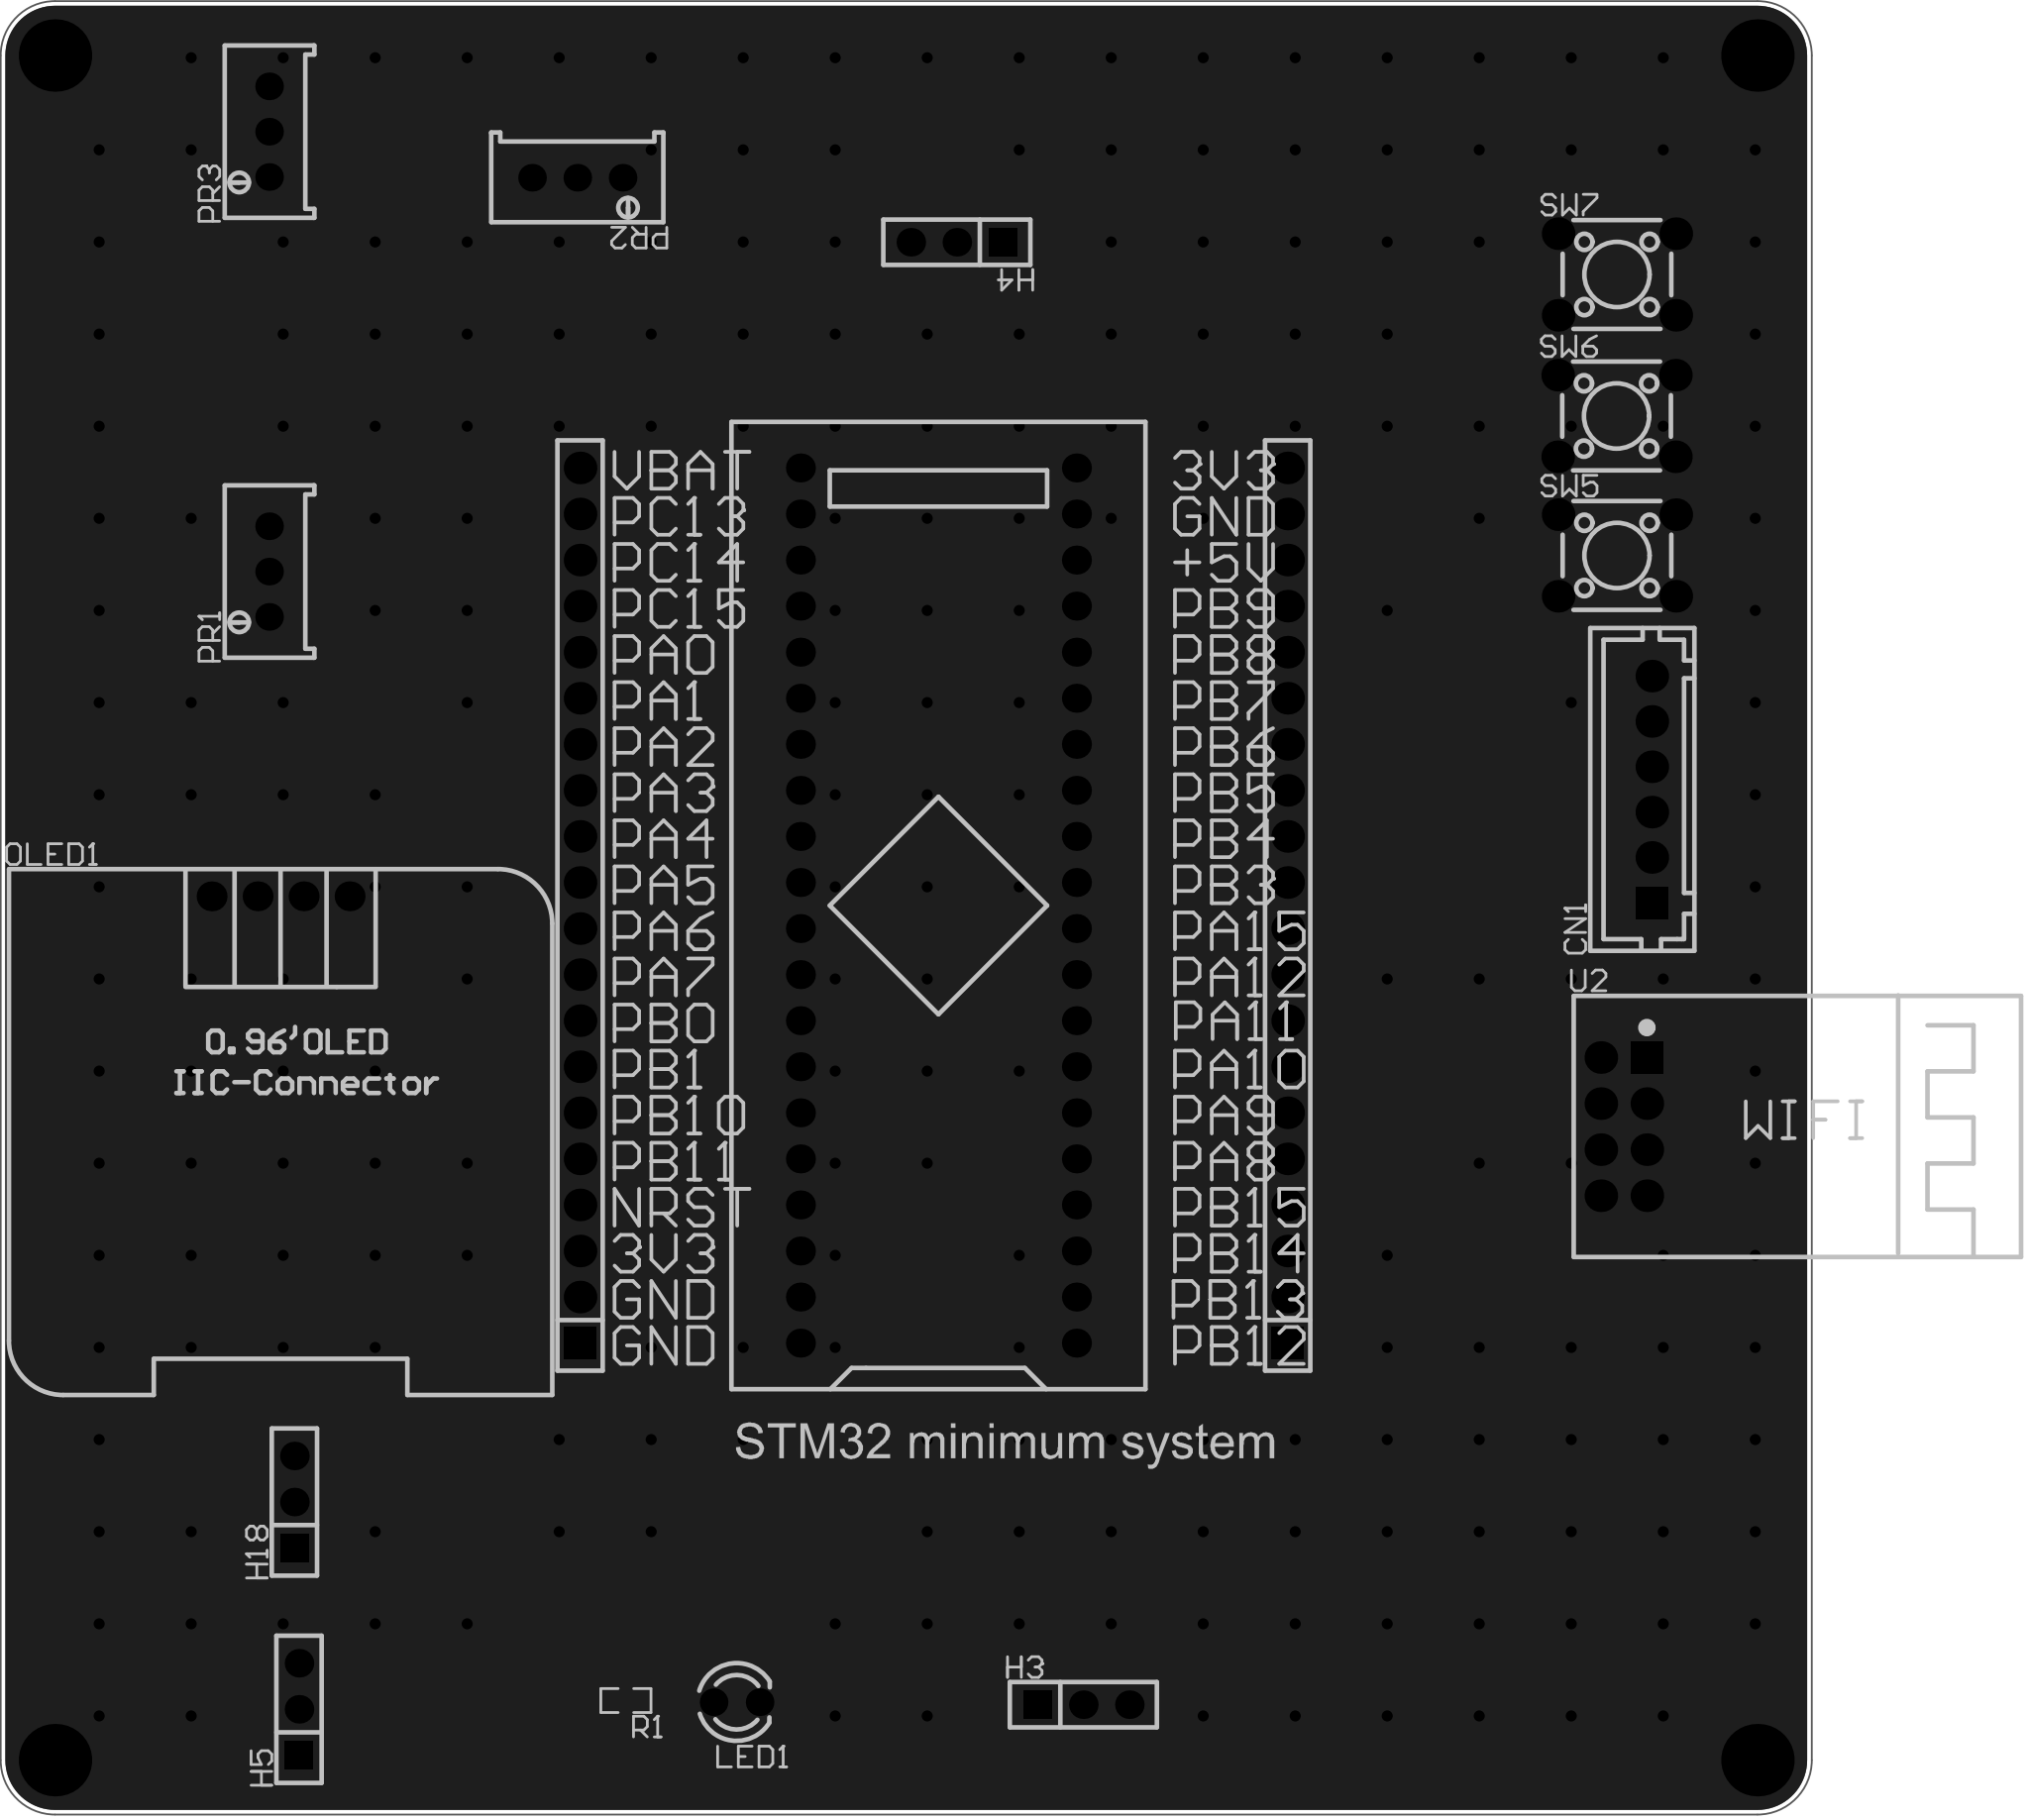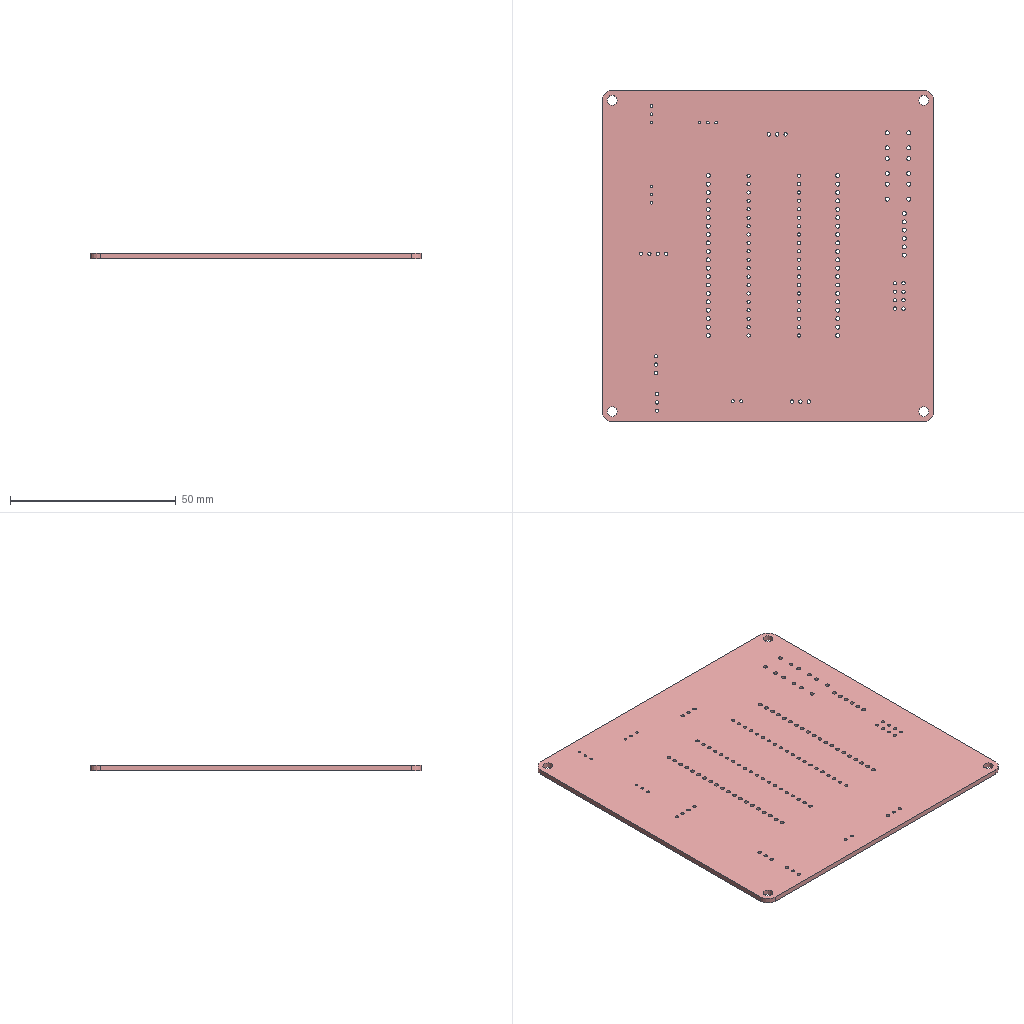Circuit board layout | Altium Designer | box 100 x 100 x 1.6 mm
Layer stack:
# Altium Designer layer stack of  (unit mm; dielectric type: 0 none, 1 core, 2 prepreg, 3 surface material)
index,name,kind,layer,copper_thickness_mm,dielectric_type,dielectric_thickness_mm,dielectric_material,dielectric_constant
0,Top Paste Mask Layer,other,,,,,,
1,Top Silkscreen Layer,other,,,,,,
2,Top Solder Mask Layer,dielectric,,,3,0.01,,3.3
3,Top Layer,copper,Top Layer,0.035,,,,
4,Dielectric1,dielectric,,,3,1.51,FR4,4.5
5,Bottom Layer,copper,Bottom Layer,0.035,,,,
6,Bottom Solder Mask Layer,dielectric,,,3,0.01,,3.3
7,Bottom Silkscreen Layer,other,,,,,,
8,Bottom Paste Mask Layer,other,,,,,,
# drill layer pairs: low layer,high layer
drill_pair,Top Layer,Bottom Layer
Part placement:
Designator,Comment,Layer,Footprint,Center-X(mm),Center-Y(mm),Rotation
U1,STM32F103C8T6-Card,TopLayer,CONN-TH_L53.3-W22.9_STM32F103C8T6-CARD,132.334,129.032,90
H1,,TopLayer,HDR-TH_20P-P2.54-V-F,151.617,129.032,90
H2,,TopLayer,HDR-TH_20P-P2.54-V-F,112.546,129.032,90
CN1,XH2.54-6PIN,TopLayer,CONN-TH_6P-P2.50-V-M_753,171.725,135.434,90
H3,,TopLayer,HDR-TH_3P-P2.54-V-F,140.335,84.963,0
H4,,TopLayer,HDR-TH_3P-P2.54-V-F,133.35,165.608,180
H5,,TopLayer,HDR-TH_3P-P2.54-V-F,97.028,84.709,90
H18,,TopLayer,HDR-TH_3P-P2.54-V-F,96.774,96.139,90
LED1,,TopLayer,LED_TH-3mm,121.191,85.099,0
OLED1,,TopLayer,0.96OLED_4P,96.012,129.54,0
PR1,10kΩ,TopLayer,R_3296,95.377,147.447,90
PR2,10kΩ,TopLayer,R_3296,112.395,169.164,180
PR3,10kΩ,TopLayer,R_3296,95.377,171.704,90
R1,300,TopLayer,R0603,115.078,85.193,180
SW5,,TopLayer,SW-TH_4P-L6.0-W6.0-P4.50-LS6.5,169.799,148.336,0
SW6,,TopLayer,SW-TH_4P-L6.0-W6.0-P4.50-LS6.5,169.776,156.028,0
SW7,,TopLayer,SW-TH_4P-L6.0-W6.0-P4.50-LS6.5,169.799,163.83,0
U2,Ai-Thinker ESP-01S ESP8266,TopLayer,WIFIM-TH_8P-L24.7-W14.4-P2.54,170.18,116.84,0
Pad and via stacks:
# Altium Designer via and pad stacks of  (unit mm). Each distinct definition once, with the count of objects using it.
# via: kind,start_layer,end_layer,hole_mm,diameter_mm,mode(0 simple;1 top-mid-bottom;2 full stack),diameter_per_layer,count,example_net
# pad: kind,layer,hole_mm,hole_type(0 round;1 square;2 slot),plating,top_size,top_shape(1 round;2 rect;3 octagon;9 rounded rect),mid_size,bottom_size,mode,footprint,size_per_layer,count,example
pad,Multi-Layer,3,0,plated,4x4,1,4x4,4x4,0,,,4,1
pad,Multi-Layer,1,0,plated,1.6x1.6,1,1.6x1.6,1.6x1.6,0,CONN-TH_L53.3-W22.9_STM32F103C8T6-CARD,,40,U1.1
pad,Multi-Layer,1.2,0,plated,1.8x1.8,2,1.8x1.8,1.8x1.8,0,HDR-TH_20P-P2.54-V-F,,2,H1.1
pad,Multi-Layer,1.2,0,plated,1.8x1.8,1,1.8x1.8,1.8x1.8,0,HDR-TH_20P-P2.54-V-F,,38,H1.2
pad,Multi-Layer,1.2,0,plated,1.8x1.8,1,1.8x1.8,1.8x1.8,0,CONN-TH_6P-P2.50-V-M_753,,5,CN1.6
pad,Multi-Layer,1.2,0,plated,1.8x1.8,2,1.8x1.8,1.8x1.8,0,CONN-TH_6P-P2.50-V-M_753,,1,CN1.1
pad,Multi-Layer,1.02,0,plated,1.575x1.575,1,1.575x1.575,1.575x1.575,0,HDR-TH_3P-P2.54-V-F,,8,H3.3
pad,Multi-Layer,1.02,0,plated,1.575x1.575,2,1.575x1.575,1.575x1.575,0,HDR-TH_3P-P2.54-V-F,,4,H3.1
pad,Multi-Layer,0.9144,0,plated,1.524x1.524,1,1.524x1.524,1.524x1.524,0,LED_TH-3mm,,2,LED1.1
pad,Multi-Layer,1,0,plated,1.65x1.65,1,1.65x1.65,1.65x1.65,0,0.96OLED_4P,,4,OLED1.4
pad,Multi-Layer,0.762,0,plated,1.524x1.524,1,1.524x1.524,1.524x1.524,0,R_3296,,9,PR1.2
pad,Multi-Layer,1.2,0,plated,1.8x1.8,1,1.8x1.8,1.8x1.8,0,SW-TH_4P-L6.0-W6.0-P4.50-LS6.5,,12,SW5.1
pad,Multi-Layer,1,0,plated,1.8x1.8,1,1.8x1.8,1.8x1.8,0,WIFIM-TH_8P-L24.7-W14.4-P2.54,,7,U2.8
pad,Multi-Layer,1,0,plated,1.8x1.8,2,1.8x1.8,1.8x1.8,0,WIFIM-TH_8P-L24.7-W14.4-P2.54,,1,U2.1
pad,Top Layer,0,0,plated,0.8065x0.864,2,0.8065x0.864,0.8065x0.864,0,R0603,,2,R1.2
via,Top Layer,Bottom Layer,0.3048,0.61,0,,228,GND
Copper pours:
name,layer,net,type(0 solid;1 hatched;2 none)
Bottom Layer-GND,Bottom Layer,GND,0
Top Layer-GND,Top Layer,GND,0